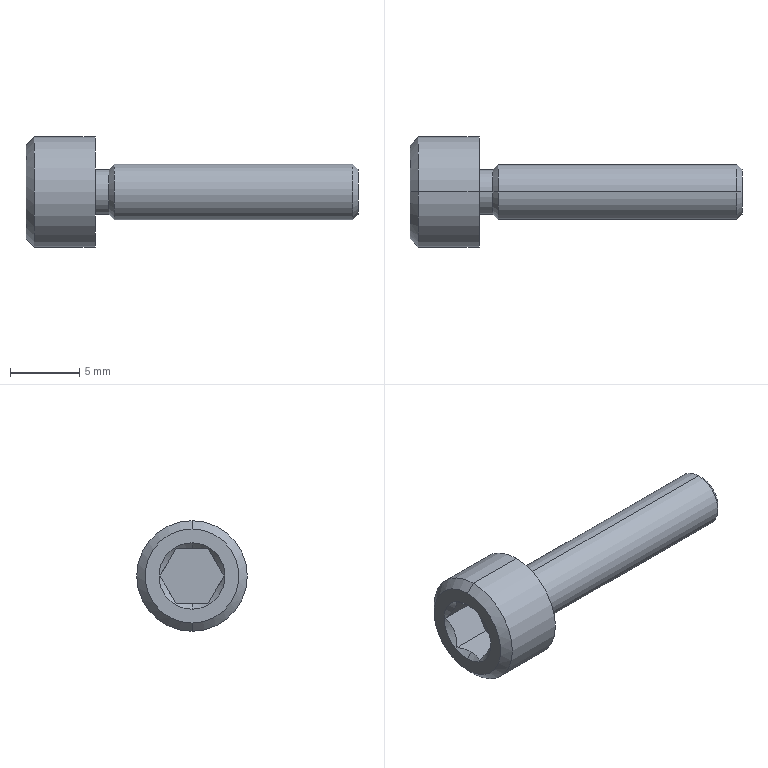Part | STEP file | LFSP35B17boltbolt | 1 solid | 24 faces | box 24 x 8 x 8 mm | volume 437.542 mm3 | plane 10 | cone 8 | cylinder 6 | commonest cylinder face diameters 3.242 x2 4 x2 8 x2